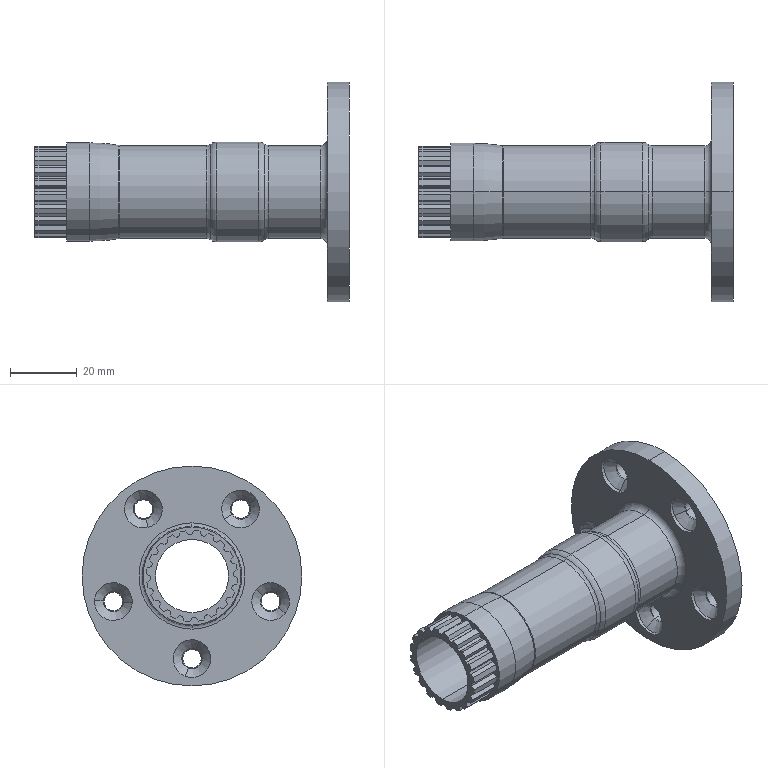Part | STEP file | Completa.sldasm-Part-3_Valor predeterminado | 1 solid | 162 faces | box 94.392 x 66 x 66 mm | volume 40484 mm3 | plane 64 | cylinder 54 | torus 22 | cone 20 | other 2 | commonest cylinder face diameters 24.944 x20 6 x10 11.34 x10 28 x4 5.596 x2 22 x2